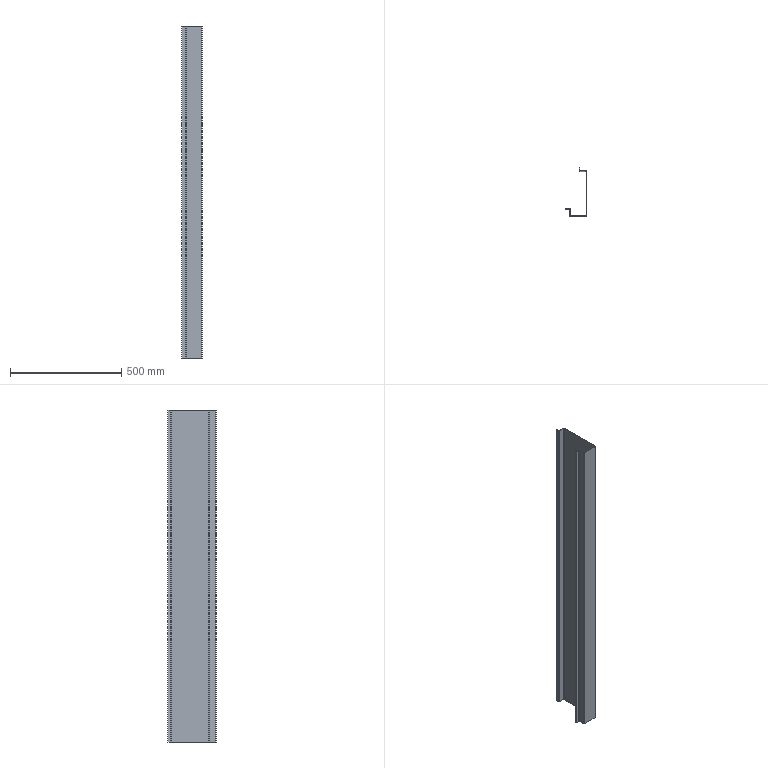Part | SolidWorks | features BaseBody 1 | 1 solid | 46 faces | box 92.2 x 216 x 1489 mm | volume 543457 mm3 | plane 36 | cylinder 10 | commonest cylinder face diameters 2 x5 4 x5
STEP:
#1=CARTESIAN_POINT('',(62.2,171.,0.));
#2=VERTEX_POINT('',#1);
#3=CARTESIAN_POINT('',(62.2,184.,0.));
#4=VERTEX_POINT('',#3);
#5=CARTESIAN_POINT('',(62.2,169.,0.));
#6=DIRECTION('',(0.,1.,0.));
#7=VECTOR('',#6,1000.);
#8=LINE('',#5,#7);
#9=EDGE_CURVE('',#2,#4,#8,.T.);
#10=ORIENTED_EDGE('',*,*,#9,.F.);
#11=CARTESIAN_POINT('',(61.2,171.,0.));
#12=VERTEX_POINT('',#11);
#13=CARTESIAN_POINT('',(62.2,171.,0.));
#14=DIRECTION('',(-1.,0.,0.));
#15=VECTOR('',#14,1000.);
#16=LINE('',#13,#15);
#17=EDGE_CURVE('',#2,#12,#16,.T.);
#18=ORIENTED_EDGE('',*,*,#17,.T.);
#19=CARTESIAN_POINT('',(61.2,184.,0.));
#20=VERTEX_POINT('',#19);
#21=CARTESIAN_POINT('',(61.2,169.,0.));
#22=DIRECTION('',(0.,1.,0.));
#23=VECTOR('',#22,1000.);
#24=LINE('',#21,#23);
#25=EDGE_CURVE('',#12,#20,#24,.T.);
#26=ORIENTED_EDGE('',*,*,#25,.T.);
#27=CARTESIAN_POINT('',(61.2,184.,0.));
#28=DIRECTION('',(1.,0.,0.));
#29=VECTOR('',#28,1000.);
#30=LINE('',#27,#29);
#31=EDGE_CURVE('',#20,#4,#30,.T.);
#32=ORIENTED_EDGE('',*,*,#31,.T.);
#33=EDGE_LOOP('',(#10,#18,#26,#32));
#34=FACE_OUTER_BOUND('',#33,.T.);
#35=CARTESIAN_POINT('',(63.2,171.,0.));
#36=DIRECTION('',(0.,0.,1.));
#37=DIRECTION('',(1.,0.,0.));
#38=AXIS2_PLACEMENT_3D('',#35,#36,#37);
#39=PLANE('',#38);
#40=ADVANCED_FACE('',(#34),#39,.F.);
#41=CARTESIAN_POINT('',(0.,-1.,1489.));
#42=VERTEX_POINT('',#41);
#43=CARTESIAN_POINT('',(18.,-1.,1489.));
#44=VERTEX_POINT('',#43);
#45=CARTESIAN_POINT('',(0.,-1.,1489.));
#46=DIRECTION('',(1.,0.,0.));
#47=VECTOR('',#46,1000.);
#48=LINE('',#45,#47);
#49=EDGE_CURVE('',#42,#44,#48,.T.);
#50=ORIENTED_EDGE('',*,*,#49,.T.);
#51=CARTESIAN_POINT('',(18.,0.,1489.));
#52=VERTEX_POINT('',#51);
#53=CARTESIAN_POINT('',(18.,-1.,1489.));
#54=DIRECTION('',(0.,1.,0.));
#55=VECTOR('',#54,1000.);
#56=LINE('',#53,#55);
#57=EDGE_CURVE('',#44,#52,#56,.T.);
#58=ORIENTED_EDGE('',*,*,#57,.T.);
#59=CARTESIAN_POINT('',(0.,0.,1489.));
#60=VERTEX_POINT('',#59);
#61=CARTESIAN_POINT('',(0.,0.,1489.));
#62=DIRECTION('',(1.,0.,0.));
#63=VECTOR('',#62,1000.);
#64=LINE('',#61,#63);
#65=EDGE_CURVE('',#60,#52,#64,.T.);
#66=ORIENTED_EDGE('',*,*,#65,.F.);
#67=CARTESIAN_POINT('',(0.,-1.,1489.));
#68=DIRECTION('',(0.,1.,0.));
#69=VECTOR('',#68,1000.);
#70=LINE('',#67,#69);
#71=EDGE_CURVE('',#42,#60,#70,.T.);
#72=ORIENTED_EDGE('',*,*,#71,.F.);
#73=EDGE_LOOP('',(#50,#58,#66,#72));
#74=FACE_OUTER_BOUND('',#73,.T.);
#75=CARTESIAN_POINT('',(63.2,171.,1489.));
#76=DIRECTION('',(0.,0.,1.));
#77=DIRECTION('',(1.,0.,0.));
#78=AXIS2_PLACEMENT_3D('',#75,#76,#77);
#79=PLANE('',#78);
#80=ADVANCED_FACE('',(#74),#79,.T.);
#81=CARTESIAN_POINT('',(63.2,170.,0.));
#82=VERTEX_POINT('',#81);
#83=CARTESIAN_POINT('',(63.2,171.,0.));
#84=DIRECTION('',(0.,0.,-1.));
#85=DIRECTION('',(1.,0.,0.));
#86=AXIS2_PLACEMENT_3D('',#83,#84,#85);
#87=CIRCLE('',#86,1.);
#88=EDGE_CURVE('',#82,#2,#87,.T.);
#89=ORIENTED_EDGE('',*,*,#88,.T.);
#90=CARTESIAN_POINT('',(62.2,171.,1489.));
#91=VERTEX_POINT('',#90);
#92=CARTESIAN_POINT('',(62.2,171.,1489.));
#93=DIRECTION('',(0.,0.,-1.));
#94=VECTOR('',#93,1000.);
#95=LINE('',#92,#94);
#96=EDGE_CURVE('',#91,#2,#95,.T.);
#97=ORIENTED_EDGE('',*,*,#96,.F.);
#98=CARTESIAN_POINT('',(63.2,170.,1489.));
#99=VERTEX_POINT('',#98);
#100=CARTESIAN_POINT('',(63.2,171.,1489.));
#101=DIRECTION('',(0.,0.,-1.));
#102=DIRECTION('',(1.,0.,0.));
#103=AXIS2_PLACEMENT_3D('',#100,#101,#102);
#104=CIRCLE('',#103,1.);
#105=EDGE_CURVE('',#99,#91,#104,.T.);
#106=ORIENTED_EDGE('',*,*,#105,.F.);
#107=CARTESIAN_POINT('',(63.2,170.,1489.));
#108=DIRECTION('',(0.,0.,-1.));
#109=VECTOR('',#108,1000.);
#110=LINE('',#107,#109);
#111=EDGE_CURVE('',#99,#82,#110,.T.);
#112=ORIENTED_EDGE('',*,*,#111,.T.);
#113=EDGE_LOOP('',(#89,#97,#106,#112));
#114=FACE_OUTER_BOUND('',#113,.T.);
#115=CARTESIAN_POINT('',(63.2,171.,1489.));
#116=DIRECTION('',(0.,0.,-1.));
#117=DIRECTION('',(-1.,0.,0.));
#118=AXIS2_PLACEMENT_3D('',#115,#116,#117);
#119=CYLINDRICAL_SURFACE('',#118,1.);
#120=ADVANCED_FACE('',(#114),#119,.F.);
#121=CARTESIAN_POINT('',(90.2,170.,0.));
#122=VERTEX_POINT('',#121);
#123=CARTESIAN_POINT('',(91.2,170.,0.));
#124=DIRECTION('',(-1.,0.,0.));
#125=VECTOR('',#124,1000.);
#126=LINE('',#123,#125);
#127=EDGE_CURVE('',#122,#82,#126,.T.);
#128=ORIENTED_EDGE('',*,*,#127,.T.);
#129=ORIENTED_EDGE('',*,*,#111,.F.);
#130=CARTESIAN_POINT('',(90.2,170.,1489.));
#131=VERTEX_POINT('',#130);
#132=CARTESIAN_POINT('',(91.2,170.,1489.));
#133=DIRECTION('',(-1.,0.,0.));
#134=VECTOR('',#133,1000.);
#135=LINE('',#132,#134);
#136=EDGE_CURVE('',#131,#99,#135,.T.);
#137=ORIENTED_EDGE('',*,*,#136,.F.);
#138=CARTESIAN_POINT('',(90.2,170.,1489.));
#139=DIRECTION('',(0.,0.,-1.));
#140=VECTOR('',#139,1000.);
#141=LINE('',#138,#140);
#142=EDGE_CURVE('',#131,#122,#141,.T.);
#143=ORIENTED_EDGE('',*,*,#142,.T.);
#144=EDGE_LOOP('',(#128,#129,#137,#143));
#145=FACE_OUTER_BOUND('',#144,.T.);
#146=CARTESIAN_POINT('',(91.2,170.,1489.));
#147=DIRECTION('',(0.,-1.,0.));
#148=DIRECTION('',(0.,0.,-1.));
#149=AXIS2_PLACEMENT_3D('',#146,#147,#148);
#150=PLANE('',#149);
#151=ADVANCED_FACE('',(#145),#150,.F.);
#152=CARTESIAN_POINT('',(92.2,168.,0.));
#153=VERTEX_POINT('',#152);
#154=CARTESIAN_POINT('',(90.2,168.,0.));
#155=DIRECTION('',(0.,0.,1.));
#156=DIRECTION('',(1.,0.,0.));
#157=AXIS2_PLACEMENT_3D('',#154,#155,#156);
#158=CIRCLE('',#157,2.);
#159=EDGE_CURVE('',#153,#122,#158,.T.);
#160=ORIENTED_EDGE('',*,*,#159,.T.);
#161=ORIENTED_EDGE('',*,*,#142,.F.);
#162=CARTESIAN_POINT('',(92.2,168.,1489.));
#163=VERTEX_POINT('',#162);
#164=CARTESIAN_POINT('',(90.2,168.,1489.));
#165=DIRECTION('',(0.,0.,1.));
#166=DIRECTION('',(1.,0.,0.));
#167=AXIS2_PLACEMENT_3D('',#164,#165,#166);
#168=CIRCLE('',#167,2.);
#169=EDGE_CURVE('',#163,#131,#168,.T.);
#170=ORIENTED_EDGE('',*,*,#169,.F.);
#171=CARTESIAN_POINT('',(92.2,168.,1489.));
#172=DIRECTION('',(0.,0.,-1.));
#173=VECTOR('',#172,1000.);
#174=LINE('',#171,#173);
#175=EDGE_CURVE('',#163,#153,#174,.T.);
#176=ORIENTED_EDGE('',*,*,#175,.T.);
#177=EDGE_LOOP('',(#160,#161,#170,#176));
#178=FACE_OUTER_BOUND('',#177,.T.);
#179=CARTESIAN_POINT('',(90.2,168.,1489.));
#180=DIRECTION('',(0.,0.,-1.));
#181=DIRECTION('',(-1.,0.,0.));
#182=AXIS2_PLACEMENT_3D('',#179,#180,#181);
#183=CYLINDRICAL_SURFACE('',#182,2.);
#184=ADVANCED_FACE('',(#178),#183,.T.);
#185=CARTESIAN_POINT('',(92.2,-30.,0.));
#186=VERTEX_POINT('',#185);
#187=CARTESIAN_POINT('',(92.2,-31.,0.));
#188=DIRECTION('',(0.,1.,0.));
#189=VECTOR('',#188,1000.);
#190=LINE('',#187,#189);
#191=EDGE_CURVE('',#186,#153,#190,.T.);
#192=ORIENTED_EDGE('',*,*,#191,.T.);
#193=ORIENTED_EDGE('',*,*,#175,.F.);
#194=CARTESIAN_POINT('',(92.2,-30.,1489.));
#195=VERTEX_POINT('',#194);
#196=CARTESIAN_POINT('',(92.2,-31.,1489.));
#197=DIRECTION('',(0.,1.,0.));
#198=VECTOR('',#197,1000.);
#199=LINE('',#196,#198);
#200=EDGE_CURVE('',#195,#163,#199,.T.);
#201=ORIENTED_EDGE('',*,*,#200,.F.);
#202=CARTESIAN_POINT('',(92.2,-30.,1489.));
#203=DIRECTION('',(0.,0.,-1.));
#204=VECTOR('',#203,1000.);
#205=LINE('',#202,#204);
#206=EDGE_CURVE('',#195,#186,#205,.T.);
#207=ORIENTED_EDGE('',*,*,#206,.T.);
#208=EDGE_LOOP('',(#192,#193,#201,#207));
#209=FACE_OUTER_BOUND('',#208,.T.);
#210=CARTESIAN_POINT('',(92.2,-31.,1489.));
#211=DIRECTION('',(-1.,0.,0.));
#212=DIRECTION('',(0.,0.,1.));
#213=AXIS2_PLACEMENT_3D('',#210,#211,#212);
#214=PLANE('',#213);
#215=ADVANCED_FACE('',(#209),#214,.F.);
#216=CARTESIAN_POINT('',(90.2,-32.,0.));
#217=VERTEX_POINT('',#216);
#218=CARTESIAN_POINT('',(90.2,-30.,0.));
#219=DIRECTION('',(0.,0.,1.));
#220=DIRECTION('',(1.,0.,0.));
#221=AXIS2_PLACEMENT_3D('',#218,#219,#220);
#222=CIRCLE('',#221,2.);
#223=EDGE_CURVE('',#217,#186,#222,.T.);
#224=ORIENTED_EDGE('',*,*,#223,.T.);
#225=ORIENTED_EDGE('',*,*,#206,.F.);
#226=CARTESIAN_POINT('',(90.2,-32.,1489.));
#227=VERTEX_POINT('',#226);
#228=CARTESIAN_POINT('',(90.2,-30.,1489.));
#229=DIRECTION('',(0.,0.,1.));
#230=DIRECTION('',(1.,0.,0.));
#231=AXIS2_PLACEMENT_3D('',#228,#229,#230);
#232=CIRCLE('',#231,2.);
#233=EDGE_CURVE('',#227,#195,#232,.T.);
#234=ORIENTED_EDGE('',*,*,#233,.F.);
#235=CARTESIAN_POINT('',(90.2,-32.,1489.));
#236=DIRECTION('',(0.,0.,-1.));
#237=VECTOR('',#236,1000.);
#238=LINE('',#235,#237);
#239=EDGE_CURVE('',#227,#217,#238,.T.);
#240=ORIENTED_EDGE('',*,*,#239,.T.);
#241=EDGE_LOOP('',(#224,#225,#234,#240));
#242=FACE_OUTER_BOUND('',#241,.T.);
#243=CARTESIAN_POINT('',(90.2,-30.,1489.));
#244=DIRECTION('',(0.,0.,-1.));
#245=DIRECTION('',(-1.,0.,0.));
#246=AXIS2_PLACEMENT_3D('',#243,#244,#245);
#247=CYLINDRICAL_SURFACE('',#246,2.);
#248=ADVANCED_FACE('',(#242),#247,.T.);
#249=CARTESIAN_POINT('',(21.,-32.,0.));
#250=VERTEX_POINT('',#249);
#251=CARTESIAN_POINT('',(20.,-32.,0.));
#252=DIRECTION('',(1.,0.,0.));
#253=VECTOR('',#252,1000.);
#254=LINE('',#251,#253);
#255=EDGE_CURVE('',#250,#217,#254,.T.);
#256=ORIENTED_EDGE('',*,*,#255,.T.);
#257=ORIENTED_EDGE('',*,*,#239,.F.);
#258=CARTESIAN_POINT('',(21.,-32.,1489.));
#259=VERTEX_POINT('',#258);
#260=CARTESIAN_POINT('',(20.,-32.,1489.));
#261=DIRECTION('',(1.,0.,0.));
#262=VECTOR('',#261,1000.);
#263=LINE('',#260,#262);
#264=EDGE_CURVE('',#259,#227,#263,.T.);
#265=ORIENTED_EDGE('',*,*,#264,.F.);
#266=CARTESIAN_POINT('',(21.,-32.,1489.));
#267=DIRECTION('',(0.,0.,-1.));
#268=VECTOR('',#267,1000.);
#269=LINE('',#266,#268);
#270=EDGE_CURVE('',#259,#250,#269,.T.);
#271=ORIENTED_EDGE('',*,*,#270,.T.);
#272=EDGE_LOOP('',(#256,#257,#265,#271));
#273=FACE_OUTER_BOUND('',#272,.T.);
#274=CARTESIAN_POINT('',(20.,-32.,1489.));
#275=DIRECTION('',(0.,1.,0.));
#276=DIRECTION('',(1.,0.,0.));
#277=AXIS2_PLACEMENT_3D('',#274,#275,#276);
#278=PLANE('',#277);
#279=ADVANCED_FACE('',(#273),#278,.F.);
#280=CARTESIAN_POINT('',(19.,-30.,0.));
#281=VERTEX_POINT('',#280);
#282=CARTESIAN_POINT('',(21.,-30.,0.));
#283=DIRECTION('',(0.,0.,1.));
#284=DIRECTION('',(1.,0.,0.));
#285=AXIS2_PLACEMENT_3D('',#282,#283,#284);
#286=CIRCLE('',#285,2.);
#287=EDGE_CURVE('',#281,#250,#286,.T.);
#288=ORIENTED_EDGE('',*,*,#287,.T.);
#289=ORIENTED_EDGE('',*,*,#270,.F.);
#290=CARTESIAN_POINT('',(19.,-30.,1489.));
#291=VERTEX_POINT('',#290);
#292=CARTESIAN_POINT('',(21.,-30.,1489.));
#293=DIRECTION('',(0.,0.,1.));
#294=DIRECTION('',(1.,0.,0.));
#295=AXIS2_PLACEMENT_3D('',#292,#293,#294);
#296=CIRCLE('',#295,2.);
#297=EDGE_CURVE('',#291,#259,#296,.T.);
#298=ORIENTED_EDGE('',*,*,#297,.F.);
#299=CARTESIAN_POINT('',(19.,-30.,1489.));
#300=DIRECTION('',(0.,0.,-1.));
#301=VECTOR('',#300,1000.);
#302=LINE('',#299,#301);
#303=EDGE_CURVE('',#291,#281,#302,.T.);
#304=ORIENTED_EDGE('',*,*,#303,.T.);
#305=EDGE_LOOP('',(#288,#289,#298,#304));
#306=FACE_OUTER_BOUND('',#305,.T.);
#307=CARTESIAN_POINT('',(21.,-30.,1489.));
#308=DIRECTION('',(0.,0.,-1.));
#309=DIRECTION('',(-1.,0.,0.));
#310=AXIS2_PLACEMENT_3D('',#307,#308,#309);
#311=CYLINDRICAL_SURFACE('',#310,2.);
#312=ADVANCED_FACE('',(#306),#311,.T.);
#313=CARTESIAN_POINT('',(19.,-2.,0.));
#314=VERTEX_POINT('',#313);
#315=CARTESIAN_POINT('',(19.,0.,0.));
#316=DIRECTION('',(0.,-1.,0.));
#317=VECTOR('',#316,1000.);
#318=LINE('',#315,#317);
#319=EDGE_CURVE('',#314,#281,#318,.T.);
#320=ORIENTED_EDGE('',*,*,#319,.T.);
#321=ORIENTED_EDGE('',*,*,#303,.F.);
#322=CARTESIAN_POINT('',(19.,-2.,1489.));
#323=VERTEX_POINT('',#322);
#324=CARTESIAN_POINT('',(19.,0.,1489.));
#325=DIRECTION('',(0.,-1.,0.));
#326=VECTOR('',#325,1000.);
#327=LINE('',#324,#326);
#328=EDGE_CURVE('',#323,#291,#327,.T.);
#329=ORIENTED_EDGE('',*,*,#328,.F.);
#330=CARTESIAN_POINT('',(19.,-2.,1489.));
#331=DIRECTION('',(0.,0.,-1.));
#332=VECTOR('',#331,1000.);
#333=LINE('',#330,#332);
#334=EDGE_CURVE('',#323,#314,#333,.T.);
#335=ORIENTED_EDGE('',*,*,#334,.T.);
#336=EDGE_LOOP('',(#320,#321,#329,#335));
#337=FACE_OUTER_BOUND('',#336,.T.);
#338=CARTESIAN_POINT('',(19.,0.,1489.));
#339=DIRECTION('',(1.,0.,0.));
#340=DIRECTION('',(0.,1.,0.));
#341=AXIS2_PLACEMENT_3D('',#338,#339,#340);
#342=PLANE('',#341);
#343=ADVANCED_FACE('',(#337),#342,.F.);
#344=CARTESIAN_POINT('',(18.,-1.,0.));
#345=VERTEX_POINT('',#344);
#346=CARTESIAN_POINT('',(18.,-2.,0.));
#347=DIRECTION('',(0.,0.,-1.));
#348=DIRECTION('',(1.,0.,0.));
#349=AXIS2_PLACEMENT_3D('',#346,#347,#348);
#350=CIRCLE('',#349,1.);
#351=EDGE_CURVE('',#345,#314,#350,.T.);
#352=ORIENTED_EDGE('',*,*,#351,.T.);
#353=ORIENTED_EDGE('',*,*,#334,.F.);
#354=CARTESIAN_POINT('',(18.,-2.,1489.));
#355=DIRECTION('',(0.,0.,-1.));
#356=DIRECTION('',(1.,0.,0.));
#357=AXIS2_PLACEMENT_3D('',#354,#355,#356);
#358=CIRCLE('',#357,1.);
#359=EDGE_CURVE('',#44,#323,#358,.T.);
#360=ORIENTED_EDGE('',*,*,#359,.F.);
#361=CARTESIAN_POINT('',(18.,-1.,1489.));
#362=DIRECTION('',(0.,0.,-1.));
#363=VECTOR('',#362,1000.);
#364=LINE('',#361,#363);
#365=EDGE_CURVE('',#44,#345,#364,.T.);
#366=ORIENTED_EDGE('',*,*,#365,.T.);
#367=EDGE_LOOP('',(#352,#353,#360,#366));
#368=FACE_OUTER_BOUND('',#367,.T.);
#369=CARTESIAN_POINT('',(18.,-2.,1489.));
#370=DIRECTION('',(0.,0.,-1.));
#371=DIRECTION('',(-1.,0.,0.));
#372=AXIS2_PLACEMENT_3D('',#369,#370,#371);
#373=CYLINDRICAL_SURFACE('',#372,1.);
#374=ADVANCED_FACE('',(#368),#373,.F.);
#375=CARTESIAN_POINT('',(0.,-1.,0.));
#376=VERTEX_POINT('',#375);
#377=CARTESIAN_POINT('',(0.,-1.,0.));
#378=DIRECTION('',(1.,0.,0.));
#379=VECTOR('',#378,1000.);
#380=LINE('',#377,#379);
#381=EDGE_CURVE('',#376,#345,#380,.T.);
#382=ORIENTED_EDGE('',*,*,#381,.T.);
#383=ORIENTED_EDGE('',*,*,#365,.F.);
#384=ORIENTED_EDGE('',*,*,#49,.F.);
#385=CARTESIAN_POINT('',(0.,-1.,1489.));
#386=DIRECTION('',(0.,0.,-1.));
#387=VECTOR('',#386,1000.);
#388=LINE('',#385,#387);
#389=EDGE_CURVE('',#42,#376,#388,.T.);
#390=ORIENTED_EDGE('',*,*,#389,.T.);
#391=EDGE_LOOP('',(#382,#383,#384,#390));
#392=FACE_OUTER_BOUND('',#391,.T.);
#393=CARTESIAN_POINT('',(0.,-1.,1489.));
#394=DIRECTION('',(0.,1.,0.));
#395=DIRECTION('',(1.,0.,0.));
#396=AXIS2_PLACEMENT_3D('',#393,#394,#395);
#397=PLANE('',#396);
#398=ADVANCED_FACE('',(#392),#397,.F.);
#399=CARTESIAN_POINT('',(0.,0.,0.));
#400=VERTEX_POINT('',#399);
#401=CARTESIAN_POINT('',(0.,-1.,0.));
#402=DIRECTION('',(0.,1.,0.));
#403=VECTOR('',#402,1000.);
#404=LINE('',#401,#403);
#405=EDGE_CURVE('',#376,#400,#404,.T.);
#406=ORIENTED_EDGE('',*,*,#405,.F.);
#407=ORIENTED_EDGE('',*,*,#389,.F.);
#408=ORIENTED_EDGE('',*,*,#71,.T.);
#409=CARTESIAN_POINT('',(0.,0.,1489.));
#410=DIRECTION('',(0.,0.,-1.));
#411=VECTOR('',#410,1000.);
#412=LINE('',#409,#411);
#413=EDGE_CURVE('',#60,#400,#412,.T.);
#414=ORIENTED_EDGE('',*,*,#413,.T.);
#415=EDGE_LOOP('',(#406,#407,#408,#414));
#416=FACE_OUTER_BOUND('',#415,.T.);
#417=CARTESIAN_POINT('',(0.,-1.,1489.));
#418=DIRECTION('',(-1.,0.,0.));
#419=DIRECTION('',(0.,0.,1.));
#420=AXIS2_PLACEMENT_3D('',#417,#418,#419);
#421=PLANE('',#420);
#422=ADVANCED_FACE('',(#416),#421,.T.);
#423=CARTESIAN_POINT('',(18.,0.,0.));
#424=VERTEX_POINT('',#423);
#425=CARTESIAN_POINT('',(0.,0.,0.));
#426=DIRECTION('',(1.,0.,0.));
#427=VECTOR('',#426,1000.);
#428=LINE('',#425,#427);
#429=EDGE_CURVE('',#400,#424,#428,.T.);
#430=ORIENTED_EDGE('',*,*,#429,.F.);
#431=ORIENTED_EDGE('',*,*,#413,.F.);
#432=ORIENTED_EDGE('',*,*,#65,.T.);
#433=CARTESIAN_POINT('',(18.,0.,1489.));
#434=DIRECTION('',(0.,0.,-1.));
#435=VECTOR('',#434,1000.);
#436=LINE('',#433,#435);
#437=EDGE_CURVE('',#52,#424,#436,.T.);
#438=ORIENTED_EDGE('',*,*,#437,.T.);
#439=EDGE_LOOP('',(#430,#431,#432,#438));
#440=FACE_OUTER_BOUND('',#439,.T.);
#441=CARTESIAN_POINT('',(0.,0.,1489.));
#442=DIRECTION('',(0.,1.,0.));
#443=DIRECTION('',(1.,0.,0.));
#444=AXIS2_PLACEMENT_3D('',#441,#442,#443);
#445=PLANE('',#444);
#446=ADVANCED_FACE('',(#440),#445,.T.);
#447=CARTESIAN_POINT('',(20.,-2.,0.));
#448=VERTEX_POINT('',#447);
#449=CARTESIAN_POINT('',(18.,-2.,0.));
#450=DIRECTION('',(0.,0.,-1.));
#451=DIRECTION('',(1.,0.,0.));
#452=AXIS2_PLACEMENT_3D('',#449,#450,#451);
#453=CIRCLE('',#452,2.);
#454=EDGE_CURVE('',#424,#448,#453,.T.);
#455=ORIENTED_EDGE('',*,*,#454,.F.);
#456=ORIENTED_EDGE('',*,*,#437,.F.);
#457=CARTESIAN_POINT('',(20.,-2.,1489.));
#458=VERTEX_POINT('',#457);
#459=CARTESIAN_POINT('',(18.,-2.,1489.));
#460=DIRECTION('',(0.,0.,-1.));
#461=DIRECTION('',(1.,0.,0.));
#462=AXIS2_PLACEMENT_3D('',#459,#460,#461);
#463=CIRCLE('',#462,2.);
#464=EDGE_CURVE('',#52,#458,#463,.T.);
#465=ORIENTED_EDGE('',*,*,#464,.T.);
#466=CARTESIAN_POINT('',(20.,-2.,1489.));
#467=DIRECTION('',(0.,0.,-1.));
#468=VECTOR('',#467,1000.);
#469=LINE('',#466,#468);
#470=EDGE_CURVE('',#458,#448,#469,.T.);
#471=ORIENTED_EDGE('',*,*,#470,.T.);
#472=EDGE_LOOP('',(#455,#456,#465,#471));
#473=FACE_OUTER_BOUND('',#472,.T.);
#474=CARTESIAN_POINT('',(18.,-2.,1489.));
#475=DIRECTION('',(0.,0.,-1.));
#476=DIRECTION('',(-1.,0.,0.));
#477=AXIS2_PLACEMENT_3D('',#474,#475,#476);
#478=CYLINDRICAL_SURFACE('',#477,2.);
#479=ADVANCED_FACE('',(#473),#478,.T.);
#480=CARTESIAN_POINT('',(20.,-30.,0.));
#481=VERTEX_POINT('',#480);
#482=CARTESIAN_POINT('',(20.,0.,0.));
#483=DIRECTION('',(0.,-1.,0.));
#484=VECTOR('',#483,1000.);
#485=LINE('',#482,#484);
#486=EDGE_CURVE('',#448,#481,#485,.T.);
#487=ORIENTED_EDGE('',*,*,#486,.F.);
#488=ORIENTED_EDGE('',*,*,#470,.F.);
#489=CARTESIAN_POINT('',(20.,-30.,1489.));
#490=VERTEX_POINT('',#489);
#491=CARTESIAN_POINT('',(20.,0.,1489.));
#492=DIRECTION('',(0.,-1.,0.));
#493=VECTOR('',#492,1000.);
#494=LINE('',#491,#493);
#495=EDGE_CURVE('',#458,#490,#494,.T.);
#496=ORIENTED_EDGE('',*,*,#495,.T.);
#497=CARTESIAN_POINT('',(20.,-30.,1489.));
#498=DIRECTION('',(0.,0.,-1.));
#499=VECTOR('',#498,1000.);
#500=LINE('',#497,#499);
#501=EDGE_CURVE('',#490,#481,#500,.T.);
#502=ORIENTED_EDGE('',*,*,#501,.T.);
#503=EDGE_LOOP('',(#487,#488,#496,#502));
#504=FACE_OUTER_BOUND('',#503,.T.);
#505=CARTESIAN_POINT('',(20.,0.,1489.));
#506=DIRECTION('',(1.,0.,0.));
#507=DIRECTION('',(0.,1.,0.));
#508=AXIS2_PLACEMENT_3D('',#505,#506,#507);
#509=PLANE('',#508);
#510=ADVANCED_FACE('',(#504),#509,.T.);
#511=CARTESIAN_POINT('',(21.,-31.,0.));
#512=VERTEX_POINT('',#511);
#513=CARTESIAN_POINT('',(21.,-30.,0.));
#514=DIRECTION('',(0.,0.,1.));
#515=DIRECTION('',(-1.,0.,0.));
#516=AXIS2_PLACEMENT_3D('',#513,#514,#515);
#517=CIRCLE('',#516,1.);
#518=EDGE_CURVE('',#481,#512,#517,.T.);
#519=ORIENTED_EDGE('',*,*,#518,.F.);
#520=ORIENTED_EDGE('',*,*,#501,.F.);
#521=CARTESIAN_POINT('',(21.,-31.,1489.));
#522=VERTEX_POINT('',#521);
#523=CARTESIAN_POINT('',(21.,-30.,1489.));
#524=DIRECTION('',(0.,0.,1.));
#525=DIRECTION('',(-1.,0.,0.));
#526=AXIS2_PLACEMENT_3D('',#523,#524,#525);
#527=CIRCLE('',#526,1.);
#528=EDGE_CURVE('',#490,#522,#527,.T.);
#529=ORIENTED_EDGE('',*,*,#528,.T.);
#530=CARTESIAN_POINT('',(21.,-31.,1489.));
#531=DIRECTION('',(0.,0.,-1.));
#532=VECTOR('',#531,1000.);
#533=LINE('',#530,#532);
#534=EDGE_CURVE('',#522,#512,#533,.T.);
#535=ORIENTED_EDGE('',*,*,#534,.T.);
#536=EDGE_LOOP('',(#519,#520,#529,#535));
#537=FACE_OUTER_BOUND('',#536,.T.);
#538=CARTESIAN_POINT('',(21.,-30.,1489.));
#539=DIRECTION('',(0.,0.,-1.));
#540=DIRECTION('',(-1.,0.,0.));
#541=AXIS2_PLACEMENT_3D('',#538,#539,#540);
#542=CYLINDRICAL_SURFACE('',#541,1.);
#543=ADVANCED_FACE('',(#537),#542,.F.);
#544=CARTESIAN_POINT('',(90.2,-31.,0.));
#545=VERTEX_POINT('',#544);
#546=CARTESIAN_POINT('',(20.,-31.,0.));
#547=DIRECTION('',(1.,0.,0.));
#548=VECTOR('',#547,1000.);
#549=LINE('',#546,#548);
#550=EDGE_CURVE('',#512,#545,#549,.T.);
#551=ORIENTED_EDGE('',*,*,#550,.F.);
#552=ORIENTED_EDGE('',*,*,#534,.F.);
#553=CARTESIAN_POINT('',(90.2,-31.,1489.));
#554=VERTEX_POINT('',#553);
#555=CARTESIAN_POINT('',(20.,-31.,1489.));
#556=DIRECTION('',(1.,0.,0.));
#557=VECTOR('',#556,1000.);
#558=LINE('',#555,#557);
#559=EDGE_CURVE('',#522,#554,#558,.T.);
#560=ORIENTED_EDGE('',*,*,#559,.T.);
#561=CARTESIAN_POINT('',(90.2,-31.,1489.));
#562=DIRECTION('',(0.,0.,-1.));
#563=VECTOR('',#562,1000.);
#564=LINE('',#561,#563);
#565=EDGE_CURVE('',#554,#545,#564,.T.);
#566=ORIENTED_EDGE('',*,*,#565,.T.);
#567=EDGE_LOOP('',(#551,#552,#560,#566));
#568=FACE_OUTER_BOUND('',#567,.T.);
#569=CARTESIAN_POINT('',(20.,-31.,1489.));
#570=DIRECTION('',(0.,1.,0.));
#571=DIRECTION('',(1.,0.,0.));
#572=AXIS2_PLACEMENT_3D('',#569,#570,#571);
#573=PLANE('',#572);
#574=ADVANCED_FACE('',(#568),#573,.T.);
#575=CARTESIAN_POINT('',(91.2,-30.,0.));
#576=VERTEX_POINT('',#575);
#577=CARTESIAN_POINT('',(90.2,-30.,0.));
#578=DIRECTION('',(0.,0.,1.));
#579=DIRECTION('',(-1.,0.,0.));
#580=AXIS2_PLACEMENT_3D('',#577,#578,#579);
#581=CIRCLE('',#580,1.);
#582=EDGE_CURVE('',#545,#576,#581,.T.);
#583=ORIENTED_EDGE('',*,*,#582,.F.);
#584=ORIENTED_EDGE('',*,*,#565,.F.);
#585=CARTESIAN_POINT('',(91.2,-30.,1489.));
#586=VERTEX_POINT('',#585);
#587=CARTESIAN_POINT('',(90.2,-30.,1489.));
#588=DIRECTION('',(0.,0.,1.));
#589=DIRECTION('',(-1.,0.,0.));
#590=AXIS2_PLACEMENT_3D('',#587,#588,#589);
#591=CIRCLE('',#590,1.);
#592=EDGE_CURVE('',#554,#586,#591,.T.);
#593=ORIENTED_EDGE('',*,*,#592,.T.);
#594=CARTESIAN_POINT('',(91.2,-30.,1489.));
#595=DIRECTION('',(0.,0.,-1.));
#596=VECTOR('',#595,1000.);
#597=LINE('',#594,#596);
#598=EDGE_CURVE('',#586,#576,#597,.T.);
#599=ORIENTED_EDGE('',*,*,#598,.T.);
#600=EDGE_LOOP('',(#583,#584,#593,#599));
#601=FACE_OUTER_BOUND('',#600,.T.);
#602=CARTESIAN_POINT('',(90.2,-30.,1489.));
#603=DIRECTION('',(0.,0.,-1.));
#604=DIRECTION('',(-1.,0.,0.));
#605=AXIS2_PLACEMENT_3D('',#602,#603,#604);
#606=CYLINDRICAL_SURFACE('',#605,1.);
#607=ADVANCED_FACE('',(#601),#606,.F.);
#608=CARTESIAN_POINT('',(91.2,168.,0.));
#609=VERTEX_POINT('',#608);
#610=CARTESIAN_POINT('',(91.2,-31.,0.));
#611=DIRECTION('',(0.,1.,0.));
#612=VECTOR('',#611,1000.);
#613=LINE('',#610,#612);
#614=EDGE_CURVE('',#576,#609,#613,.T.);
#615=ORIENTED_EDGE('',*,*,#614,.F.);
#616=ORIENTED_EDGE('',*,*,#598,.F.);
#617=CARTESIAN_POINT('',(91.2,168.,1489.));
#618=VERTEX_POINT('',#617);
#619=CARTESIAN_POINT('',(91.2,-31.,1489.));
#620=DIRECTION('',(0.,1.,0.));
#621=VECTOR('',#620,1000.);
#622=LINE('',#619,#621);
#623=EDGE_CURVE('',#586,#618,#622,.T.);
#624=ORIENTED_EDGE('',*,*,#623,.T.);
#625=CARTESIAN_POINT('',(91.2,168.,1489.));
#626=DIRECTION('',(0.,0.,-1.));
#627=VECTOR('',#626,1000.);
#628=LINE('',#625,#627);
#629=EDGE_CURVE('',#618,#609,#628,.T.);
#630=ORIENTED_EDGE('',*,*,#629,.T.);
#631=EDGE_LOOP('',(#615,#616,#624,#630));
#632=FACE_OUTER_BOUND('',#631,.T.);
#633=CARTESIAN_POINT('',(91.2,-31.,1489.));
#634=DIRECTION('',(-1.,0.,0.));
#635=DIRECTION('',(0.,0.,1.));
#636=AXIS2_PLACEMENT_3D('',#633,#634,#635);
#637=PLANE('',#636);
#638=ADVANCED_FACE('',(#632),#637,.T.);
#639=CARTESIAN_POINT('',(90.2,169.,0.));
#640=VERTEX_POINT('',#639);
#641=CARTESIAN_POINT('',(90.2,168.,0.));
#642=DIRECTION('',(0.,0.,1.));
#643=DIRECTION('',(-1.,0.,0.));
#644=AXIS2_PLACEMENT_3D('',#641,#642,#643);
#645=CIRCLE('',#644,1.);
#646=EDGE_CURVE('',#609,#640,#645,.T.);
#647=ORIENTED_EDGE('',*,*,#646,.F.);
#648=ORIENTED_EDGE('',*,*,#629,.F.);
#649=CARTESIAN_POINT('',(90.2,169.,1489.));
#650=VERTEX_POINT('',#649);
#651=CARTESIAN_POINT('',(90.2,168.,1489.));
#652=DIRECTION('',(0.,0.,1.));
#653=DIRECTION('',(-1.,0.,0.));
#654=AXIS2_PLACEMENT_3D('',#651,#652,#653);
#655=CIRCLE('',#654,1.);
#656=EDGE_CURVE('',#618,#650,#655,.T.);
#657=ORIENTED_EDGE('',*,*,#656,.T.);
#658=CARTESIAN_POINT('',(90.2,169.,1489.));
#659=DIRECTION('',(0.,0.,-1.));
#660=VECTOR('',#659,1000.);
#661=LINE('',#658,#660);
#662=EDGE_CURVE('',#650,#640,#661,.T.);
#663=ORIENTED_EDGE('',*,*,#662,.T.);
#664=EDGE_LOOP('',(#647,#648,#657,#663));
#665=FACE_OUTER_BOUND('',#664,.T.);
#666=CARTESIAN_POINT('',(90.2,168.,1489.));
#667=DIRECTION('',(0.,0.,-1.));
#668=DIRECTION('',(-1.,0.,0.));
#669=AXIS2_PLACEMENT_3D('',#666,#667,#668);
#670=CYLINDRICAL_SURFACE('',#669,1.);
#671=ADVANCED_FACE('',(#665),#670,.F.);
#672=CARTESIAN_POINT('',(63.2,169.,0.));
#673=VERTEX_POINT('',#672);
#674=CARTESIAN_POINT('',(91.2,169.,0.));
#675=DIRECTION('',(-1.,0.,0.));
#676=VECTOR('',#675,1000.);
#677=LINE('',#674,#676);
#678=EDGE_CURVE('',#640,#673,#677,.T.);
#679=ORIENTED_EDGE('',*,*,#678,.F.);
#680=ORIENTED_EDGE('',*,*,#662,.F.);
#681=CARTESIAN_POINT('',(63.2,169.,1489.));
#682=VERTEX_POINT('',#681);
#683=CARTESIAN_POINT('',(91.2,169.,1489.));
#684=DIRECTION('',(-1.,0.,0.));
#685=VECTOR('',#684,1000.);
#686=LINE('',#683,#685);
#687=EDGE_CURVE('',#650,#682,#686,.T.);
#688=ORIENTED_EDGE('',*,*,#687,.T.);
#689=CARTESIAN_POINT('',(63.2,169.,1489.));
#690=DIRECTION('',(0.,0.,-1.));
#691=VECTOR('',#690,1000.);
#692=LINE('',#689,#691);
#693=EDGE_CURVE('',#682,#673,#692,.T.);
#694=ORIENTED_EDGE('',*,*,#693,.T.);
#695=EDGE_LOOP('',(#679,#680,#688,#694));
#696=FACE_OUTER_BOUND('',#695,.T.);
#697=CARTESIAN_POINT('',(91.2,169.,1489.));
#698=DIRECTION('',(0.,-1.,0.));
#699=DIRECTION('',(0.,0.,-1.));
#700=AXIS2_PLACEMENT_3D('',#697,#698,#699);
#701=PLANE('',#700);
#702=ADVANCED_FACE('',(#696),#701,.T.);
#703=CARTESIAN_POINT('',(63.2,171.,0.));
#704=DIRECTION('',(0.,0.,-1.));
#705=DIRECTION('',(1.,0.,0.));
#706=AXIS2_PLACEMENT_3D('',#703,#704,#705);
#707=CIRCLE('',#706,2.);
#708=EDGE_CURVE('',#673,#12,#707,.T.);
#709=ORIENTED_EDGE('',*,*,#708,.F.);
#710=ORIENTED_EDGE('',*,*,#693,.F.);
#711=CARTESIAN_POINT('',(61.2,171.,1489.));
#712=VERTEX_POINT('',#711);
#713=CARTESIAN_POINT('',(63.2,171.,1489.));
#714=DIRECTION('',(0.,0.,-1.));
#715=DIRECTION('',(1.,0.,0.));
#716=AXIS2_PLACEMENT_3D('',#713,#714,#715);
#717=CIRCLE('',#716,2.);
#718=EDGE_CURVE('',#682,#712,#717,.T.);
#719=ORIENTED_EDGE('',*,*,#718,.T.);
#720=CARTESIAN_POINT('',(61.2,171.,1489.));
#721=DIRECTION('',(0.,0.,-1.));
#722=VECTOR('',#721,1000.);
#723=LINE('',#720,#722);
#724=EDGE_CURVE('',#712,#12,#723,.T.);
#725=ORIENTED_EDGE('',*,*,#724,.T.);
#726=EDGE_LOOP('',(#709,#710,#719,#725));
#727=FACE_OUTER_BOUND('',#726,.T.);
#728=CARTESIAN_POINT('',(63.2,171.,1489.));
#729=DIRECTION('',(0.,0.,-1.));
#730=DIRECTION('',(-1.,0.,0.));
#731=AXIS2_PLACEMENT_3D('',#728,#729,#730);
#732=CYLINDRICAL_SURFACE('',#731,2.);
#733=ADVANCED_FACE('',(#727),#732,.T.);
#734=ORIENTED_EDGE('',*,*,#25,.F.);
#735=ORIENTED_EDGE('',*,*,#724,.F.);
#736=CARTESIAN_POINT('',(61.2,184.,1489.));
#737=VERTEX_POINT('',#736);
#738=CARTESIAN_POINT('',(61.2,169.,1489.));
#739=DIRECTION('',(0.,1.,0.));
#740=VECTOR('',#739,1000.);
#741=LINE('',#738,#740);
#742=EDGE_CURVE('',#712,#737,#741,.T.);
#743=ORIENTED_EDGE('',*,*,#742,.T.);
#744=CARTESIAN_POINT('',(61.2,184.,1489.));
#745=DIRECTION('',(0.,0.,-1.));
#746=VECTOR('',#745,1000.);
#747=LINE('',#744,#746);
#748=EDGE_CURVE('',#737,#20,#747,.T.);
#749=ORIENTED_EDGE('',*,*,#748,.T.);
#750=EDGE_LOOP('',(#734,#735,#743,#749));
#751=FACE_OUTER_BOUND('',#750,.T.);
#752=CARTESIAN_POINT('',(61.2,169.,1489.));
#753=DIRECTION('',(-1.,0.,0.));
#754=DIRECTION('',(0.,0.,1.));
#755=AXIS2_PLACEMENT_3D('',#752,#753,#754);
#756=PLANE('',#755);
#757=ADVANCED_FACE('',(#751),#756,.T.);
#758=ORIENTED_EDGE('',*,*,#31,.F.);
#759=ORIENTED_EDGE('',*,*,#748,.F.);
#760=CARTESIAN_POINT('',(62.2,184.,1489.));
#761=VERTEX_POINT('',#760);
#762=CARTESIAN_POINT('',(61.2,184.,1489.));
#763=DIRECTION('',(1.,0.,0.));
#764=VECTOR('',#763,1000.);
#765=LINE('',#762,#764);
#766=EDGE_CURVE('',#737,#761,#765,.T.);
#767=ORIENTED_EDGE('',*,*,#766,.T.);
#768=CARTESIAN_POINT('',(62.2,184.,1489.));
#769=DIRECTION('',(0.,0.,-1.));
#770=VECTOR('',#769,1000.);
#771=LINE('',#768,#770);
#772=EDGE_CURVE('',#761,#4,#771,.T.);
#773=ORIENTED_EDGE('',*,*,#772,.T.);
#774=EDGE_LOOP('',(#758,#759,#767,#773));
#775=FACE_OUTER_BOUND('',#774,.T.);
#776=CARTESIAN_POINT('',(61.2,184.,1489.));
#777=DIRECTION('',(0.,1.,0.));
#778=DIRECTION('',(1.,0.,0.));
#779=AXIS2_PLACEMENT_3D('',#776,#777,#778);
#780=PLANE('',#779);
#781=ADVANCED_FACE('',(#775),#780,.T.);
#782=ORIENTED_EDGE('',*,*,#9,.T.);
#783=ORIENTED_EDGE('',*,*,#772,.F.);
#784=CARTESIAN_POINT('',(62.2,169.,1489.));
#785=DIRECTION('',(0.,1.,0.));
#786=VECTOR('',#785,1000.);
#787=LINE('',#784,#786);
#788=EDGE_CURVE('',#91,#761,#787,.T.);
#789=ORIENTED_EDGE('',*,*,#788,.F.);
#790=ORIENTED_EDGE('',*,*,#96,.T.);
#791=EDGE_LOOP('',(#782,#783,#789,#790));
#792=FACE_OUTER_BOUND('',#791,.T.);
#793=CARTESIAN_POINT('',(62.2,169.,1489.));
#794=DIRECTION('',(-1.,0.,0.));
#795=DIRECTION('',(0.,0.,1.));
#796=AXIS2_PLACEMENT_3D('',#793,#794,#795);
#797=PLANE('',#796);
#798=ADVANCED_FACE('',(#792),#797,.F.);
#799=ORIENTED_EDGE('',*,*,#678,.T.);
#800=CARTESIAN_POINT('',(63.2,169.,0.));
#801=DIRECTION('',(0.,1.,0.));
#802=VECTOR('',#801,1000.);
#803=LINE('',#800,#802);
#804=EDGE_CURVE('',#673,#82,#803,.T.);
#805=ORIENTED_EDGE('',*,*,#804,.T.);
#806=ORIENTED_EDGE('',*,*,#127,.F.);
#807=CARTESIAN_POINT('',(90.2,170.,0.));
#808=DIRECTION('',(0.,-1.,0.));
#809=VECTOR('',#808,1000.);
#810=LINE('',#807,#809);
#811=EDGE_CURVE('',#122,#640,#810,.T.);
#812=ORIENTED_EDGE('',*,*,#811,.T.);
#813=EDGE_LOOP('',(#799,#805,#806,#812));
#814=FACE_OUTER_BOUND('',#813,.T.);
#815=CARTESIAN_POINT('',(62.2,171.,0.));
#816=DIRECTION('',(0.,0.,-1.));
#817=DIRECTION('',(0.,-1.,0.));
#818=AXIS2_PLACEMENT_3D('',#815,#816,#817);
#819=PLANE('',#818);
#820=ADVANCED_FACE('',(#814),#819,.T.);
#821=ORIENTED_EDGE('',*,*,#804,.F.);
#822=ORIENTED_EDGE('',*,*,#708,.T.);
#823=ORIENTED_EDGE('',*,*,#17,.F.);
#824=ORIENTED_EDGE('',*,*,#88,.F.);
#825=EDGE_LOOP('',(#821,#822,#823,#824));
#826=FACE_OUTER_BOUND('',#825,.T.);
#827=CARTESIAN_POINT('',(63.2,169.,0.));
#828=DIRECTION('',(0.,0.,-1.));
#829=DIRECTION('',(0.,-1.,0.));
#830=AXIS2_PLACEMENT_3D('',#827,#828,#829);
#831=PLANE('',#830);
#832=ADVANCED_FACE('',(#826),#831,.T.);
#833=ORIENTED_EDGE('',*,*,#742,.F.);
#834=CARTESIAN_POINT('',(61.2,171.,1489.));
#835=DIRECTION('',(1.,0.,0.));
#836=VECTOR('',#835,1000.);
#837=LINE('',#834,#836);
#838=EDGE_CURVE('',#712,#91,#837,.T.);
#839=ORIENTED_EDGE('',*,*,#838,.T.);
#840=ORIENTED_EDGE('',*,*,#788,.T.);
#841=ORIENTED_EDGE('',*,*,#766,.F.);
#842=EDGE_LOOP('',(#833,#839,#840,#841));
#843=FACE_OUTER_BOUND('',#842,.T.);
#844=CARTESIAN_POINT('',(63.2,170.,1489.));
#845=DIRECTION('',(0.,0.,1.));
#846=DIRECTION('',(1.,0.,0.));
#847=AXIS2_PLACEMENT_3D('',#844,#845,#846);
#848=PLANE('',#847);
#849=ADVANCED_FACE('',(#843),#848,.T.);
#850=ORIENTED_EDGE('',*,*,#838,.F.);
#851=ORIENTED_EDGE('',*,*,#718,.F.);
#852=CARTESIAN_POINT('',(63.2,170.,1489.));
#853=DIRECTION('',(0.,-1.,0.));
#854=VECTOR('',#853,1000.);
#855=LINE('',#852,#854);
#856=EDGE_CURVE('',#99,#682,#855,.T.);
#857=ORIENTED_EDGE('',*,*,#856,.F.);
#858=ORIENTED_EDGE('',*,*,#105,.T.);
#859=EDGE_LOOP('',(#850,#851,#857,#858));
#860=FACE_OUTER_BOUND('',#859,.T.);
#861=CARTESIAN_POINT('',(61.2,171.,1489.));
#862=DIRECTION('',(0.,0.,1.));
#863=DIRECTION('',(1.,0.,0.));
#864=AXIS2_PLACEMENT_3D('',#861,#862,#863);
#865=PLANE('',#864);
#866=ADVANCED_FACE('',(#860),#865,.T.);
#867=ORIENTED_EDGE('',*,*,#614,.T.);
#868=CARTESIAN_POINT('',(91.2,168.,0.));
#869=DIRECTION('',(1.,0.,0.));
#870=VECTOR('',#869,1000.);
#871=LINE('',#868,#870);
#872=EDGE_CURVE('',#609,#153,#871,.T.);
#873=ORIENTED_EDGE('',*,*,#872,.T.);
#874=ORIENTED_EDGE('',*,*,#191,.F.);
#875=CARTESIAN_POINT('',(92.2,-30.,0.));
#876=DIRECTION('',(-1.,0.,0.));
#877=VECTOR('',#876,1000.);
#878=LINE('',#875,#877);
#879=EDGE_CURVE('',#186,#576,#878,.T.);
#880=ORIENTED_EDGE('',*,*,#879,.T.);
#881=EDGE_LOOP('',(#867,#873,#874,#880));
#882=FACE_OUTER_BOUND('',#881,.T.);
#883=CARTESIAN_POINT('',(90.2,170.,0.));
#884=DIRECTION('',(0.,0.,-1.));
#885=DIRECTION('',(0.,-1.,0.));
#886=AXIS2_PLACEMENT_3D('',#883,#884,#885);
#887=PLANE('',#886);
#888=ADVANCED_FACE('',(#882),#887,.T.);
#889=ORIENTED_EDGE('',*,*,#872,.F.);
#890=ORIENTED_EDGE('',*,*,#646,.T.);
#891=ORIENTED_EDGE('',*,*,#811,.F.);
#892=ORIENTED_EDGE('',*,*,#159,.F.);
#893=EDGE_LOOP('',(#889,#890,#891,#892));
#894=FACE_OUTER_BOUND('',#893,.T.);
#895=CARTESIAN_POINT('',(91.2,168.,0.));
#896=DIRECTION('',(0.,0.,-1.));
#897=DIRECTION('',(0.,-1.,0.));
#898=AXIS2_PLACEMENT_3D('',#895,#896,#897);
#899=PLANE('',#898);
#900=ADVANCED_FACE('',(#894),#899,.T.);
#901=ORIENTED_EDGE('',*,*,#687,.F.);
#902=CARTESIAN_POINT('',(90.2,169.,1489.));
#903=DIRECTION('',(0.,1.,0.));
#904=VECTOR('',#903,1000.);
#905=LINE('',#902,#904);
#906=EDGE_CURVE('',#650,#131,#905,.T.);
#907=ORIENTED_EDGE('',*,*,#906,.T.);
#908=ORIENTED_EDGE('',*,*,#136,.T.);
#909=ORIENTED_EDGE('',*,*,#856,.T.);
#910=EDGE_LOOP('',(#901,#907,#908,#909));
#911=FACE_OUTER_BOUND('',#910,.T.);
#912=CARTESIAN_POINT('',(92.2,168.,1489.));
#913=DIRECTION('',(0.,0.,1.));
#914=DIRECTION('',(1.,0.,0.));
#915=AXIS2_PLACEMENT_3D('',#912,#913,#914);
#916=PLANE('',#915);
#917=ADVANCED_FACE('',(#911),#916,.T.);
#918=ORIENTED_EDGE('',*,*,#906,.F.);
#919=ORIENTED_EDGE('',*,*,#656,.F.);
#920=CARTESIAN_POINT('',(92.2,168.,1489.));
#921=DIRECTION('',(-1.,0.,0.));
#922=VECTOR('',#921,1000.);
#923=LINE('',#920,#922);
#924=EDGE_CURVE('',#163,#618,#923,.T.);
#925=ORIENTED_EDGE('',*,*,#924,.F.);
#926=ORIENTED_EDGE('',*,*,#169,.T.);
#927=EDGE_LOOP('',(#918,#919,#925,#926));
#928=FACE_OUTER_BOUND('',#927,.T.);
#929=CARTESIAN_POINT('',(90.2,169.,1489.));
#930=DIRECTION('',(0.,0.,1.));
#931=DIRECTION('',(1.,0.,0.));
#932=AXIS2_PLACEMENT_3D('',#929,#930,#931);
#933=PLANE('',#932);
#934=ADVANCED_FACE('',(#928),#933,.T.);
#935=ORIENTED_EDGE('',*,*,#550,.T.);
#936=CARTESIAN_POINT('',(90.2,-31.,0.));
#937=DIRECTION('',(0.,-1.,0.));
#938=VECTOR('',#937,1000.);
#939=LINE('',#936,#938);
#940=EDGE_CURVE('',#545,#217,#939,.T.);
#941=ORIENTED_EDGE('',*,*,#940,.T.);
#942=ORIENTED_EDGE('',*,*,#255,.F.);
#943=CARTESIAN_POINT('',(21.,-32.,0.));
#944=DIRECTION('',(0.,1.,0.));
#945=VECTOR('',#944,1000.);
#946=LINE('',#943,#945);
#947=EDGE_CURVE('',#250,#512,#946,.T.);
#948=ORIENTED_EDGE('',*,*,#947,.T.);
#949=EDGE_LOOP('',(#935,#941,#942,#948));
#950=FACE_OUTER_BOUND('',#949,.T.);
#951=CARTESIAN_POINT('',(92.2,-30.,0.));
#952=DIRECTION('',(0.,0.,-1.));
#953=DIRECTION('',(0.,-1.,0.));
#954=AXIS2_PLACEMENT_3D('',#951,#952,#953);
#955=PLANE('',#954);
#956=ADVANCED_FACE('',(#950),#955,.T.);
#957=ORIENTED_EDGE('',*,*,#940,.F.);
#958=ORIENTED_EDGE('',*,*,#582,.T.);
#959=ORIENTED_EDGE('',*,*,#879,.F.);
#960=ORIENTED_EDGE('',*,*,#223,.F.);
#961=EDGE_LOOP('',(#957,#958,#959,#960));
#962=FACE_OUTER_BOUND('',#961,.T.);
#963=CARTESIAN_POINT('',(90.2,-31.,0.));
#964=DIRECTION('',(0.,0.,-1.));
#965=DIRECTION('',(0.,-1.,0.));
#966=AXIS2_PLACEMENT_3D('',#963,#964,#965);
#967=PLANE('',#966);
#968=ADVANCED_FACE('',(#962),#967,.T.);
#969=ORIENTED_EDGE('',*,*,#623,.F.);
#970=CARTESIAN_POINT('',(91.2,-30.,1489.));
#971=DIRECTION('',(1.,0.,0.));
#972=VECTOR('',#971,1000.);
#973=LINE('',#970,#972);
#974=EDGE_CURVE('',#586,#195,#973,.T.);
#975=ORIENTED_EDGE('',*,*,#974,.T.);
#976=ORIENTED_EDGE('',*,*,#200,.T.);
#977=ORIENTED_EDGE('',*,*,#924,.T.);
#978=EDGE_LOOP('',(#969,#975,#976,#977));
#979=FACE_OUTER_BOUND('',#978,.T.);
#980=CARTESIAN_POINT('',(90.2,-32.,1489.));
#981=DIRECTION('',(0.,0.,1.));
#982=DIRECTION('',(1.,0.,0.));
#983=AXIS2_PLACEMENT_3D('',#980,#981,#982);
#984=PLANE('',#983);
#985=ADVANCED_FACE('',(#979),#984,.T.);
#986=ORIENTED_EDGE('',*,*,#974,.F.);
#987=ORIENTED_EDGE('',*,*,#592,.F.);
#988=CARTESIAN_POINT('',(90.2,-32.,1489.));
#989=DIRECTION('',(0.,1.,0.));
#990=VECTOR('',#989,1000.);
#991=LINE('',#988,#990);
#992=EDGE_CURVE('',#227,#554,#991,.T.);
#993=ORIENTED_EDGE('',*,*,#992,.F.);
#994=ORIENTED_EDGE('',*,*,#233,.T.);
#995=EDGE_LOOP('',(#986,#987,#993,#994));
#996=FACE_OUTER_BOUND('',#995,.T.);
#997=CARTESIAN_POINT('',(91.2,-30.,1489.));
#998=DIRECTION('',(0.,0.,1.));
#999=DIRECTION('',(1.,0.,0.));
#1000=AXIS2_PLACEMENT_3D('',#997,#998,#999);
#1001=PLANE('',#1000);
#1002=ADVANCED_FACE('',(#996),#1001,.T.);
#1003=ORIENTED_EDGE('',*,*,#486,.T.);
#1004=CARTESIAN_POINT('',(20.,-30.,0.));
#1005=DIRECTION('',(-1.,0.,0.));
#1006=VECTOR('',#1005,1000.);
#1007=LINE('',#1004,#1006);
#1008=EDGE_CURVE('',#481,#281,#1007,.T.);
#1009=ORIENTED_EDGE('',*,*,#1008,.T.);
#1010=ORIENTED_EDGE('',*,*,#319,.F.);
#1011=CARTESIAN_POINT('',(19.,-2.,0.));
#1012=DIRECTION('',(1.,0.,0.));
#1013=VECTOR('',#1012,1000.);
#1014=LINE('',#1011,#1013);
#1015=EDGE_CURVE('',#314,#448,#1014,.T.);
#1016=ORIENTED_EDGE('',*,*,#1015,.T.);
#1017=EDGE_LOOP('',(#1003,#1009,#1010,#1016));
#1018=FACE_OUTER_BOUND('',#1017,.T.);
#1019=CARTESIAN_POINT('',(21.,-32.,0.));
#1020=DIRECTION('',(0.,0.,-1.));
#1021=DIRECTION('',(0.,-1.,0.));
#1022=AXIS2_PLACEMENT_3D('',#1019,#1020,#1021);
#1023=PLANE('',#1022);
#1024=ADVANCED_FACE('',(#1018),#1023,.T.);
#1025=ORIENTED_EDGE('',*,*,#1008,.F.);
#1026=ORIENTED_EDGE('',*,*,#518,.T.);
#1027=ORIENTED_EDGE('',*,*,#947,.F.);
#1028=ORIENTED_EDGE('',*,*,#287,.F.);
#1029=EDGE_LOOP('',(#1025,#1026,#1027,#1028));
#1030=FACE_OUTER_BOUND('',#1029,.T.);
#1031=CARTESIAN_POINT('',(20.,-30.,0.));
#1032=DIRECTION('',(0.,0.,-1.));
#1033=DIRECTION('',(0.,-1.,0.));
#1034=AXIS2_PLACEMENT_3D('',#1031,#1032,#1033);
#1035=PLANE('',#1034);
#1036=ADVANCED_FACE('',(#1030),#1035,.T.);
#1037=ORIENTED_EDGE('',*,*,#559,.F.);
#1038=CARTESIAN_POINT('',(21.,-31.,1489.));
#1039=DIRECTION('',(0.,-1.,0.));
#1040=VECTOR('',#1039,1000.);
#1041=LINE('',#1038,#1040);
#1042=EDGE_CURVE('',#522,#259,#1041,.T.);
#1043=ORIENTED_EDGE('',*,*,#1042,.T.);
#1044=ORIENTED_EDGE('',*,*,#264,.T.);
#1045=ORIENTED_EDGE('',*,*,#992,.T.);
#1046=EDGE_LOOP('',(#1037,#1043,#1044,#1045));
#1047=FACE_OUTER_BOUND('',#1046,.T.);
#1048=CARTESIAN_POINT('',(19.,-30.,1489.));
#1049=DIRECTION('',(0.,0.,1.));
#1050=DIRECTION('',(1.,0.,0.));
#1051=AXIS2_PLACEMENT_3D('',#1048,#1049,#1050);
#1052=PLANE('',#1051);
#1053=ADVANCED_FACE('',(#1047),#1052,.T.);
#1054=ORIENTED_EDGE('',*,*,#1042,.F.);
#1055=ORIENTED_EDGE('',*,*,#528,.F.);
#1056=CARTESIAN_POINT('',(19.,-30.,1489.));
#1057=DIRECTION('',(1.,0.,0.));
#1058=VECTOR('',#1057,1000.);
#1059=LINE('',#1056,#1058);
#1060=EDGE_CURVE('',#291,#490,#1059,.T.);
#1061=ORIENTED_EDGE('',*,*,#1060,.F.);
#1062=ORIENTED_EDGE('',*,*,#297,.T.);
#1063=EDGE_LOOP('',(#1054,#1055,#1061,#1062));
#1064=FACE_OUTER_BOUND('',#1063,.T.);
#1065=CARTESIAN_POINT('',(21.,-31.,1489.));
#1066=DIRECTION('',(0.,0.,1.));
#1067=DIRECTION('',(1.,0.,0.));
#1068=AXIS2_PLACEMENT_3D('',#1065,#1066,#1067);
#1069=PLANE('',#1068);
#1070=ADVANCED_FACE('',(#1064),#1069,.T.);
#1071=ORIENTED_EDGE('',*,*,#429,.T.);
#1072=CARTESIAN_POINT('',(18.,0.,0.));
#1073=DIRECTION('',(0.,-1.,0.));
#1074=VECTOR('',#1073,1000.);
#1075=LINE('',#1072,#1074);
#1076=EDGE_CURVE('',#424,#345,#1075,.T.);
#1077=ORIENTED_EDGE('',*,*,#1076,.T.);
#1078=ORIENTED_EDGE('',*,*,#381,.F.);
#1079=ORIENTED_EDGE('',*,*,#405,.T.);
#1080=EDGE_LOOP('',(#1071,#1077,#1078,#1079));
#1081=FACE_OUTER_BOUND('',#1080,.T.);
#1082=CARTESIAN_POINT('',(19.,-2.,0.));
#1083=DIRECTION('',(0.,0.,-1.));
#1084=DIRECTION('',(0.,-1.,0.));
#1085=AXIS2_PLACEMENT_3D('',#1082,#1083,#1084);
#1086=PLANE('',#1085);
#1087=ADVANCED_FACE('',(#1081),#1086,.T.);
#1088=ORIENTED_EDGE('',*,*,#1076,.F.);
#1089=ORIENTED_EDGE('',*,*,#454,.T.);
#1090=ORIENTED_EDGE('',*,*,#1015,.F.);
#1091=ORIENTED_EDGE('',*,*,#351,.F.);
#1092=EDGE_LOOP('',(#1088,#1089,#1090,#1091));
#1093=FACE_OUTER_BOUND('',#1092,.T.);
#1094=CARTESIAN_POINT('',(18.,0.,0.));
#1095=DIRECTION('',(0.,0.,-1.));
#1096=DIRECTION('',(0.,-1.,0.));
#1097=AXIS2_PLACEMENT_3D('',#1094,#1095,#1096);
#1098=PLANE('',#1097);
#1099=ADVANCED_FACE('',(#1093),#1098,.T.);
#1100=ORIENTED_EDGE('',*,*,#495,.F.);
#1101=CARTESIAN_POINT('',(20.,-2.,1489.));
#1102=DIRECTION('',(-1.,0.,0.));
#1103=VECTOR('',#1102,1000.);
#1104=LINE('',#1101,#1103);
#1105=EDGE_CURVE('',#458,#323,#1104,.T.);
#1106=ORIENTED_EDGE('',*,*,#1105,.T.);
#1107=ORIENTED_EDGE('',*,*,#328,.T.);
#1108=ORIENTED_EDGE('',*,*,#1060,.T.);
#1109=EDGE_LOOP('',(#1100,#1106,#1107,#1108));
#1110=FACE_OUTER_BOUND('',#1109,.T.);
#1111=CARTESIAN_POINT('',(18.,-1.,1489.));
#1112=DIRECTION('',(0.,0.,1.));
#1113=DIRECTION('',(1.,0.,0.));
#1114=AXIS2_PLACEMENT_3D('',#1111,#1112,#1113);
#1115=PLANE('',#1114);
#1116=ADVANCED_FACE('',(#1110),#1115,.T.);
#1117=ORIENTED_EDGE('',*,*,#1105,.F.);
#1118=ORIENTED_EDGE('',*,*,#464,.F.);
#1119=ORIENTED_EDGE('',*,*,#57,.F.);
#1120=ORIENTED_EDGE('',*,*,#359,.T.);
#1121=EDGE_LOOP('',(#1117,#1118,#1119,#1120));
#1122=FACE_OUTER_BOUND('',#1121,.T.);
#1123=CARTESIAN_POINT('',(20.,-2.,1489.));
#1124=DIRECTION('',(0.,0.,1.));
#1125=DIRECTION('',(1.,0.,0.));
#1126=AXIS2_PLACEMENT_3D('',#1123,#1124,#1125);
#1127=PLANE('',#1126);
#1128=ADVANCED_FACE('',(#1122),#1127,.T.);
#1129=CLOSED_SHELL('',(#40,#80,#120,#151,#184,#215,#248,#279,#312,#343,#374,#398,#422,#446,#479,#510,#543,#574,#607,#638,#671,#702,#733,#757,#781,#798,#820,#832,#849,#866,#888,#900,#917,#934,#956,#968,#985,#1002,#1024,#1036,#1053,#1070,#1087,#1099,#1116,#1128));
#1130=MANIFOLD_SOLID_BREP('',#1129);
#1131=CARTESIAN_POINT('',(0.,0.,0.));
#1132=DIRECTION('',(0.,0.,1.));
#1133=DIRECTION('',(1.,0.,0.));
#1134=AXIS2_PLACEMENT_3D('',#1131,#1132,#1133);
#1135=(LENGTH_UNIT()NAMED_UNIT(*)SI_UNIT(.MILLI.,.METRE.));
#1136=UNCERTAINTY_MEASURE_WITH_UNIT(LENGTH_MEASURE(0.00001),#1135,'','');
#1137=(NAMED_UNIT(*)PLANE_ANGLE_UNIT()SI_UNIT($,.RADIAN.));
#1138=(NAMED_UNIT(*)SI_UNIT($,.STERADIAN.)SOLID_ANGLE_UNIT());
#1139=(GEOMETRIC_REPRESENTATION_CONTEXT(3)GLOBAL_UNCERTAINTY_ASSIGNED_CONTEXT((#1136))GLOBAL_UNIT_ASSIGNED_CONTEXT((#1135,#1137,#1138))REPRESENTATION_CONTEXT('',''));
#1140=ADVANCED_BREP_SHAPE_REPRESENTATION('',(#1130,#1134),#1139);